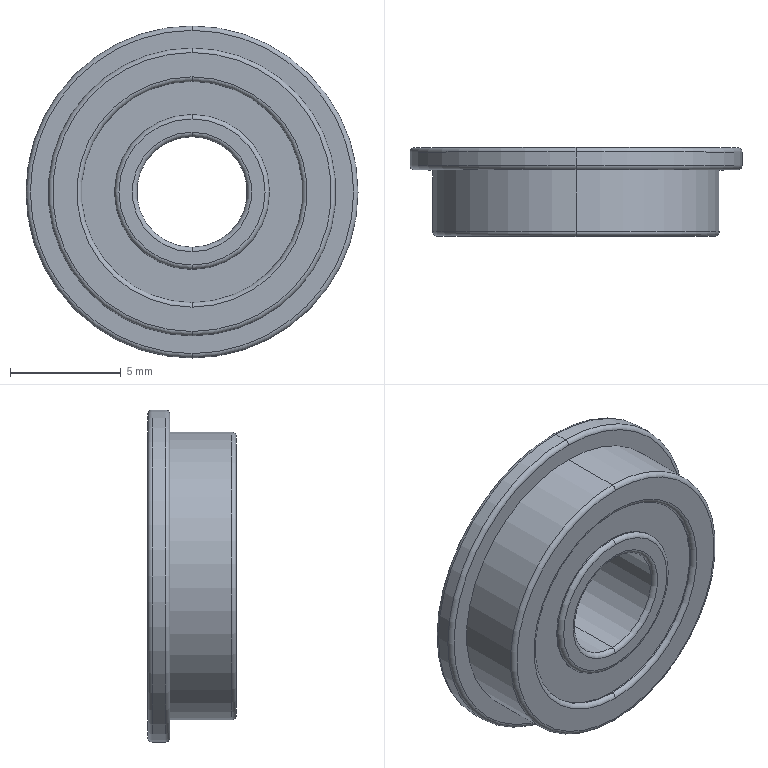Part | NX | features BREP 1 | 1 solid | 39 faces | box 15 x 4 x 15 mm | volume 474 mm3 | torus 18 | cylinder 14 | plane 7 | commonest cylinder face diameters 7 x4 10 x4 5 x2 13 x2 15 x2
STEP:
#1=CARTESIAN_POINT('',(0.,3.8,2.5));
#2=VERTEX_POINT('',#1);
#3=CARTESIAN_POINT('',(0.,4.,2.7));
#4=VERTEX_POINT('',#3);
#5=CARTESIAN_POINT('',(0.,3.8,2.7));
#6=DIRECTION('',(1.,0.,0.));
#7=DIRECTION('',(0.,0.,-1.));
#8=AXIS2_PLACEMENT_3D('',#5,#6,#7);
#9=CIRCLE('',#8,0.2);
#10=EDGE_CURVE('',#2,#4,#9,.T.);
#11=ORIENTED_EDGE('',*,*,#10,.F.);
#12=CARTESIAN_POINT('',(0.,3.8,-2.5));
#13=VERTEX_POINT('',#12);
#14=CARTESIAN_POINT('',(0.,3.8,0.));
#15=DIRECTION('',(0.,1.,0.));
#16=DIRECTION('',(0.,0.,-1.));
#17=AXIS2_PLACEMENT_3D('',#14,#15,#16);
#18=CIRCLE('',#17,2.5);
#19=EDGE_CURVE('',#13,#2,#18,.T.);
#20=ORIENTED_EDGE('',*,*,#19,.F.);
#21=CARTESIAN_POINT('',(0.,4.,-2.7));
#22=VERTEX_POINT('',#21);
#23=CARTESIAN_POINT('',(0.,3.8,-2.7));
#24=DIRECTION('',(-1.,0.,0.));
#25=DIRECTION('',(0.,0.,1.));
#26=AXIS2_PLACEMENT_3D('',#23,#24,#25);
#27=CIRCLE('',#26,0.2);
#28=EDGE_CURVE('',#13,#22,#27,.T.);
#29=ORIENTED_EDGE('',*,*,#28,.T.);
#30=CARTESIAN_POINT('',(0.,4.,0.));
#31=DIRECTION('',(0.,-1.,0.));
#32=DIRECTION('',(0.,0.,-1.));
#33=AXIS2_PLACEMENT_3D('',#30,#31,#32);
#34=CIRCLE('',#33,2.7);
#35=EDGE_CURVE('',#4,#22,#34,.T.);
#36=ORIENTED_EDGE('',*,*,#35,.F.);
#37=EDGE_LOOP('',(#11,#20,#29,#36));
#38=FACE_BOUND('',#37,.T.);
#39=CARTESIAN_POINT('',(0.,3.8,0.));
#40=DIRECTION('',(0.,-1.,0.));
#41=DIRECTION('',(0.,0.,-1.));
#42=AXIS2_PLACEMENT_3D('',#39,#40,#41);
#43=TOROIDAL_SURFACE('',#42,2.7,0.2);
#44=ADVANCED_FACE('',(#38),#43,.T.);
#45=CARTESIAN_POINT('',(0.,4.,3.3));
#46=VERTEX_POINT('',#45);
#47=CARTESIAN_POINT('',(0.,3.8,3.5));
#48=VERTEX_POINT('',#47);
#49=CARTESIAN_POINT('',(0.,3.8,3.3));
#50=DIRECTION('',(1.,0.,0.));
#51=DIRECTION('',(0.,0.,-1.));
#52=AXIS2_PLACEMENT_3D('',#49,#50,#51);
#53=CIRCLE('',#52,0.2);
#54=EDGE_CURVE('',#46,#48,#53,.T.);
#55=ORIENTED_EDGE('',*,*,#54,.F.);
#56=CARTESIAN_POINT('',(0.,4.,-3.3));
#57=VERTEX_POINT('',#56);
#58=CARTESIAN_POINT('',(0.,4.,0.));
#59=DIRECTION('',(0.,1.,0.));
#60=DIRECTION('',(0.,0.,-1.));
#61=AXIS2_PLACEMENT_3D('',#58,#59,#60);
#62=CIRCLE('',#61,3.3);
#63=EDGE_CURVE('',#57,#46,#62,.T.);
#64=ORIENTED_EDGE('',*,*,#63,.F.);
#65=CARTESIAN_POINT('',(0.,3.8,-3.5));
#66=VERTEX_POINT('',#65);
#67=CARTESIAN_POINT('',(0.,3.8,-3.3));
#68=DIRECTION('',(-1.,0.,0.));
#69=DIRECTION('',(0.,0.,1.));
#70=AXIS2_PLACEMENT_3D('',#67,#68,#69);
#71=CIRCLE('',#70,0.2);
#72=EDGE_CURVE('',#57,#66,#71,.T.);
#73=ORIENTED_EDGE('',*,*,#72,.T.);
#74=CARTESIAN_POINT('',(0.,3.8,0.));
#75=DIRECTION('',(0.,-1.,0.));
#76=DIRECTION('',(0.,0.,-1.));
#77=AXIS2_PLACEMENT_3D('',#74,#75,#76);
#78=CIRCLE('',#77,3.5);
#79=EDGE_CURVE('',#48,#66,#78,.T.);
#80=ORIENTED_EDGE('',*,*,#79,.F.);
#81=EDGE_LOOP('',(#55,#64,#73,#80));
#82=FACE_BOUND('',#81,.T.);
#83=CARTESIAN_POINT('',(0.,3.8,0.));
#84=DIRECTION('',(0.,-1.,0.));
#85=DIRECTION('',(0.,0.,-1.));
#86=AXIS2_PLACEMENT_3D('',#83,#84,#85);
#87=TOROIDAL_SURFACE('',#86,3.3,0.2);
#88=ADVANCED_FACE('',(#82),#87,.T.);
#89=CARTESIAN_POINT('',(0.,3.8,5.));
#90=VERTEX_POINT('',#89);
#91=CARTESIAN_POINT('',(0.,4.,5.2));
#92=VERTEX_POINT('',#91);
#93=CARTESIAN_POINT('',(0.,3.8,5.2));
#94=DIRECTION('',(1.,0.,0.));
#95=DIRECTION('',(0.,0.,-1.));
#96=AXIS2_PLACEMENT_3D('',#93,#94,#95);
#97=CIRCLE('',#96,0.2);
#98=EDGE_CURVE('',#90,#92,#97,.T.);
#99=ORIENTED_EDGE('',*,*,#98,.F.);
#100=CARTESIAN_POINT('',(0.,3.8,-5.));
#101=VERTEX_POINT('',#100);
#102=CARTESIAN_POINT('',(0.,3.8,0.));
#103=DIRECTION('',(0.,1.,0.));
#104=DIRECTION('',(0.,0.,-1.));
#105=AXIS2_PLACEMENT_3D('',#102,#103,#104);
#106=CIRCLE('',#105,5.);
#107=EDGE_CURVE('',#101,#90,#106,.T.);
#108=ORIENTED_EDGE('',*,*,#107,.F.);
#109=CARTESIAN_POINT('',(0.,4.,-5.2));
#110=VERTEX_POINT('',#109);
#111=CARTESIAN_POINT('',(0.,3.8,-5.2));
#112=DIRECTION('',(-1.,0.,0.));
#113=DIRECTION('',(0.,0.,1.));
#114=AXIS2_PLACEMENT_3D('',#111,#112,#113);
#115=CIRCLE('',#114,0.2);
#116=EDGE_CURVE('',#101,#110,#115,.T.);
#117=ORIENTED_EDGE('',*,*,#116,.T.);
#118=CARTESIAN_POINT('',(0.,4.,0.));
#119=DIRECTION('',(0.,-1.,0.));
#120=DIRECTION('',(0.,0.,-1.));
#121=AXIS2_PLACEMENT_3D('',#118,#119,#120);
#122=CIRCLE('',#121,5.2);
#123=EDGE_CURVE('',#92,#110,#122,.T.);
#124=ORIENTED_EDGE('',*,*,#123,.F.);
#125=EDGE_LOOP('',(#99,#108,#117,#124));
#126=FACE_BOUND('',#125,.T.);
#127=CARTESIAN_POINT('',(0.,3.8,0.));
#128=DIRECTION('',(0.,-1.,0.));
#129=DIRECTION('',(0.,0.,-1.));
#130=AXIS2_PLACEMENT_3D('',#127,#128,#129);
#131=TOROIDAL_SURFACE('',#130,5.2,0.2);
#132=ADVANCED_FACE('',(#126),#131,.T.);
#133=CARTESIAN_POINT('',(0.,4.,7.3));
#134=VERTEX_POINT('',#133);
#135=CARTESIAN_POINT('',(0.,3.8,7.5));
#136=VERTEX_POINT('',#135);
#137=CARTESIAN_POINT('',(0.,3.8,7.3));
#138=DIRECTION('',(1.,0.,0.));
#139=DIRECTION('',(0.,0.,-1.));
#140=AXIS2_PLACEMENT_3D('',#137,#138,#139);
#141=CIRCLE('',#140,0.2);
#142=EDGE_CURVE('',#134,#136,#141,.T.);
#143=ORIENTED_EDGE('',*,*,#142,.F.);
#144=CARTESIAN_POINT('',(0.,4.,-7.3));
#145=VERTEX_POINT('',#144);
#146=CARTESIAN_POINT('',(0.,4.,0.));
#147=DIRECTION('',(0.,1.,0.));
#148=DIRECTION('',(0.,0.,-1.));
#149=AXIS2_PLACEMENT_3D('',#146,#147,#148);
#150=CIRCLE('',#149,7.3);
#151=EDGE_CURVE('',#145,#134,#150,.T.);
#152=ORIENTED_EDGE('',*,*,#151,.F.);
#153=CARTESIAN_POINT('',(0.,3.8,-7.5));
#154=VERTEX_POINT('',#153);
#155=CARTESIAN_POINT('',(0.,3.8,-7.3));
#156=DIRECTION('',(-1.,0.,0.));
#157=DIRECTION('',(0.,0.,1.));
#158=AXIS2_PLACEMENT_3D('',#155,#156,#157);
#159=CIRCLE('',#158,0.2);
#160=EDGE_CURVE('',#145,#154,#159,.T.);
#161=ORIENTED_EDGE('',*,*,#160,.T.);
#162=CARTESIAN_POINT('',(0.,3.8,0.));
#163=DIRECTION('',(0.,-1.,0.));
#164=DIRECTION('',(0.,0.,-1.));
#165=AXIS2_PLACEMENT_3D('',#162,#163,#164);
#166=CIRCLE('',#165,7.5);
#167=EDGE_CURVE('',#136,#154,#166,.T.);
#168=ORIENTED_EDGE('',*,*,#167,.F.);
#169=EDGE_LOOP('',(#143,#152,#161,#168));
#170=FACE_BOUND('',#169,.T.);
#171=CARTESIAN_POINT('',(0.,3.8,0.));
#172=DIRECTION('',(0.,-1.,0.));
#173=DIRECTION('',(0.,0.,-1.));
#174=AXIS2_PLACEMENT_3D('',#171,#172,#173);
#175=TOROIDAL_SURFACE('',#174,7.3,0.2);
#176=ADVANCED_FACE('',(#170),#175,.T.);
#177=CARTESIAN_POINT('',(0.,3.2,-7.5));
#178=VERTEX_POINT('',#177);
#179=CARTESIAN_POINT('',(0.,3.,-7.3));
#180=VERTEX_POINT('',#179);
#181=CARTESIAN_POINT('',(0.,3.2,-7.3));
#182=DIRECTION('',(1.,0.,0.));
#183=DIRECTION('',(0.,0.,-1.));
#184=AXIS2_PLACEMENT_3D('',#181,#182,#183);
#185=CIRCLE('',#184,0.2);
#186=EDGE_CURVE('',#178,#180,#185,.F.);
#187=ORIENTED_EDGE('',*,*,#186,.T.);
#188=CARTESIAN_POINT('',(0.,3.,7.3));
#189=VERTEX_POINT('',#188);
#190=CARTESIAN_POINT('',(0.,3.,0.));
#191=DIRECTION('',(0.,-1.,0.));
#192=DIRECTION('',(0.,0.,1.));
#193=AXIS2_PLACEMENT_3D('',#190,#191,#192);
#194=CIRCLE('',#193,7.3);
#195=EDGE_CURVE('',#189,#180,#194,.T.);
#196=ORIENTED_EDGE('',*,*,#195,.F.);
#197=CARTESIAN_POINT('',(0.,3.2,7.5));
#198=VERTEX_POINT('',#197);
#199=CARTESIAN_POINT('',(0.,3.2,7.3));
#200=DIRECTION('',(-1.,0.,0.));
#201=DIRECTION('',(0.,0.,1.));
#202=AXIS2_PLACEMENT_3D('',#199,#200,#201);
#203=CIRCLE('',#202,0.2);
#204=EDGE_CURVE('',#198,#189,#203,.F.);
#205=ORIENTED_EDGE('',*,*,#204,.F.);
#206=CARTESIAN_POINT('',(0.,3.2,0.));
#207=DIRECTION('',(0.,1.,0.));
#208=DIRECTION('',(0.,0.,1.));
#209=AXIS2_PLACEMENT_3D('',#206,#207,#208);
#210=CIRCLE('',#209,7.5);
#211=EDGE_CURVE('',#178,#198,#210,.T.);
#212=ORIENTED_EDGE('',*,*,#211,.F.);
#213=EDGE_LOOP('',(#187,#196,#205,#212));
#214=FACE_BOUND('',#213,.T.);
#215=CARTESIAN_POINT('',(0.,3.2,0.));
#216=DIRECTION('',(0.,1.,0.));
#217=DIRECTION('',(0.,0.,1.));
#218=AXIS2_PLACEMENT_3D('',#215,#216,#217);
#219=TOROIDAL_SURFACE('',#218,7.3,0.2);
#220=ADVANCED_FACE('',(#214),#219,.T.);
#221=CARTESIAN_POINT('',(0.,0.2,-6.5));
#222=VERTEX_POINT('',#221);
#223=CARTESIAN_POINT('',(0.,0.,-6.3));
#224=VERTEX_POINT('',#223);
#225=CARTESIAN_POINT('',(0.,0.2,-6.3));
#226=DIRECTION('',(1.,0.,0.));
#227=DIRECTION('',(0.,0.,-1.));
#228=AXIS2_PLACEMENT_3D('',#225,#226,#227);
#229=CIRCLE('',#228,0.2);
#230=EDGE_CURVE('',#222,#224,#229,.F.);
#231=ORIENTED_EDGE('',*,*,#230,.T.);
#232=CARTESIAN_POINT('',(0.,0.,6.3));
#233=VERTEX_POINT('',#232);
#234=CARTESIAN_POINT('',(0.,0.,0.));
#235=DIRECTION('',(0.,-1.,0.));
#236=DIRECTION('',(0.,0.,1.));
#237=AXIS2_PLACEMENT_3D('',#234,#235,#236);
#238=CIRCLE('',#237,6.3);
#239=EDGE_CURVE('',#233,#224,#238,.T.);
#240=ORIENTED_EDGE('',*,*,#239,.F.);
#241=CARTESIAN_POINT('',(0.,0.2,6.5));
#242=VERTEX_POINT('',#241);
#243=CARTESIAN_POINT('',(0.,0.2,6.3));
#244=DIRECTION('',(-1.,0.,0.));
#245=DIRECTION('',(0.,0.,1.));
#246=AXIS2_PLACEMENT_3D('',#243,#244,#245);
#247=CIRCLE('',#246,0.2);
#248=EDGE_CURVE('',#242,#233,#247,.F.);
#249=ORIENTED_EDGE('',*,*,#248,.F.);
#250=CARTESIAN_POINT('',(0.,0.2,0.));
#251=DIRECTION('',(0.,1.,0.));
#252=DIRECTION('',(0.,0.,1.));
#253=AXIS2_PLACEMENT_3D('',#250,#251,#252);
#254=CIRCLE('',#253,6.5);
#255=EDGE_CURVE('',#222,#242,#254,.T.);
#256=ORIENTED_EDGE('',*,*,#255,.F.);
#257=EDGE_LOOP('',(#231,#240,#249,#256));
#258=FACE_BOUND('',#257,.T.);
#259=CARTESIAN_POINT('',(0.,0.2,0.));
#260=DIRECTION('',(0.,1.,0.));
#261=DIRECTION('',(0.,0.,1.));
#262=AXIS2_PLACEMENT_3D('',#259,#260,#261);
#263=TOROIDAL_SURFACE('',#262,6.3,0.2);
#264=ADVANCED_FACE('',(#258),#263,.T.);
#265=CARTESIAN_POINT('',(0.,0.,-5.2));
#266=VERTEX_POINT('',#265);
#267=CARTESIAN_POINT('',(0.,0.2,-5.));
#268=VERTEX_POINT('',#267);
#269=CARTESIAN_POINT('',(0.,0.2,-5.2));
#270=DIRECTION('',(1.,0.,0.));
#271=DIRECTION('',(0.,0.,-1.));
#272=AXIS2_PLACEMENT_3D('',#269,#270,#271);
#273=CIRCLE('',#272,0.2);
#274=EDGE_CURVE('',#266,#268,#273,.F.);
#275=ORIENTED_EDGE('',*,*,#274,.T.);
#276=CARTESIAN_POINT('',(0.,0.2,5.));
#277=VERTEX_POINT('',#276);
#278=CARTESIAN_POINT('',(0.,0.2,0.));
#279=DIRECTION('',(0.,-1.,0.));
#280=DIRECTION('',(0.,0.,1.));
#281=AXIS2_PLACEMENT_3D('',#278,#279,#280);
#282=CIRCLE('',#281,5.);
#283=EDGE_CURVE('',#277,#268,#282,.T.);
#284=ORIENTED_EDGE('',*,*,#283,.F.);
#285=CARTESIAN_POINT('',(0.,0.,5.2));
#286=VERTEX_POINT('',#285);
#287=CARTESIAN_POINT('',(0.,0.2,5.2));
#288=DIRECTION('',(-1.,0.,0.));
#289=DIRECTION('',(0.,0.,1.));
#290=AXIS2_PLACEMENT_3D('',#287,#288,#289);
#291=CIRCLE('',#290,0.2);
#292=EDGE_CURVE('',#286,#277,#291,.F.);
#293=ORIENTED_EDGE('',*,*,#292,.F.);
#294=CARTESIAN_POINT('',(0.,0.,0.));
#295=DIRECTION('',(0.,1.,0.));
#296=DIRECTION('',(0.,0.,1.));
#297=AXIS2_PLACEMENT_3D('',#294,#295,#296);
#298=CIRCLE('',#297,5.2);
#299=EDGE_CURVE('',#266,#286,#298,.T.);
#300=ORIENTED_EDGE('',*,*,#299,.F.);
#301=EDGE_LOOP('',(#275,#284,#293,#300));
#302=FACE_BOUND('',#301,.T.);
#303=CARTESIAN_POINT('',(0.,0.2,0.));
#304=DIRECTION('',(0.,1.,0.));
#305=DIRECTION('',(0.,0.,1.));
#306=AXIS2_PLACEMENT_3D('',#303,#304,#305);
#307=TOROIDAL_SURFACE('',#306,5.2,0.2);
#308=ADVANCED_FACE('',(#302),#307,.T.);
#309=CARTESIAN_POINT('',(0.,0.2,-3.5));
#310=VERTEX_POINT('',#309);
#311=CARTESIAN_POINT('',(0.,0.,-3.3));
#312=VERTEX_POINT('',#311);
#313=CARTESIAN_POINT('',(0.,0.2,-3.3));
#314=DIRECTION('',(1.,0.,0.));
#315=DIRECTION('',(0.,0.,-1.));
#316=AXIS2_PLACEMENT_3D('',#313,#314,#315);
#317=CIRCLE('',#316,0.2);
#318=EDGE_CURVE('',#310,#312,#317,.F.);
#319=ORIENTED_EDGE('',*,*,#318,.T.);
#320=CARTESIAN_POINT('',(0.,0.,3.3));
#321=VERTEX_POINT('',#320);
#322=CARTESIAN_POINT('',(0.,0.,0.));
#323=DIRECTION('',(0.,-1.,0.));
#324=DIRECTION('',(0.,0.,1.));
#325=AXIS2_PLACEMENT_3D('',#322,#323,#324);
#326=CIRCLE('',#325,3.3);
#327=EDGE_CURVE('',#321,#312,#326,.T.);
#328=ORIENTED_EDGE('',*,*,#327,.F.);
#329=CARTESIAN_POINT('',(0.,0.2,3.5));
#330=VERTEX_POINT('',#329);
#331=CARTESIAN_POINT('',(0.,0.2,3.3));
#332=DIRECTION('',(-1.,0.,0.));
#333=DIRECTION('',(0.,0.,1.));
#334=AXIS2_PLACEMENT_3D('',#331,#332,#333);
#335=CIRCLE('',#334,0.2);
#336=EDGE_CURVE('',#330,#321,#335,.F.);
#337=ORIENTED_EDGE('',*,*,#336,.F.);
#338=CARTESIAN_POINT('',(0.,0.2,0.));
#339=DIRECTION('',(0.,1.,0.));
#340=DIRECTION('',(0.,0.,1.));
#341=AXIS2_PLACEMENT_3D('',#338,#339,#340);
#342=CIRCLE('',#341,3.5);
#343=EDGE_CURVE('',#310,#330,#342,.T.);
#344=ORIENTED_EDGE('',*,*,#343,.F.);
#345=EDGE_LOOP('',(#319,#328,#337,#344));
#346=FACE_BOUND('',#345,.T.);
#347=CARTESIAN_POINT('',(0.,0.2,0.));
#348=DIRECTION('',(0.,1.,0.));
#349=DIRECTION('',(0.,0.,1.));
#350=AXIS2_PLACEMENT_3D('',#347,#348,#349);
#351=TOROIDAL_SURFACE('',#350,3.3,0.2);
#352=ADVANCED_FACE('',(#346),#351,.T.);
#353=CARTESIAN_POINT('',(0.,0.,-2.7));
#354=VERTEX_POINT('',#353);
#355=CARTESIAN_POINT('',(0.,0.2,-2.5));
#356=VERTEX_POINT('',#355);
#357=CARTESIAN_POINT('',(0.,0.2,-2.7));
#358=DIRECTION('',(1.,0.,0.));
#359=DIRECTION('',(0.,0.,-1.));
#360=AXIS2_PLACEMENT_3D('',#357,#358,#359);
#361=CIRCLE('',#360,0.2);
#362=EDGE_CURVE('',#354,#356,#361,.F.);
#363=ORIENTED_EDGE('',*,*,#362,.T.);
#364=CARTESIAN_POINT('',(0.,0.2,2.5));
#365=VERTEX_POINT('',#364);
#366=CARTESIAN_POINT('',(0.,0.2,0.));
#367=DIRECTION('',(0.,-1.,0.));
#368=DIRECTION('',(0.,0.,1.));
#369=AXIS2_PLACEMENT_3D('',#366,#367,#368);
#370=CIRCLE('',#369,2.5);
#371=EDGE_CURVE('',#365,#356,#370,.T.);
#372=ORIENTED_EDGE('',*,*,#371,.F.);
#373=CARTESIAN_POINT('',(0.,0.,2.7));
#374=VERTEX_POINT('',#373);
#375=CARTESIAN_POINT('',(0.,0.2,2.7));
#376=DIRECTION('',(-1.,0.,0.));
#377=DIRECTION('',(0.,0.,1.));
#378=AXIS2_PLACEMENT_3D('',#375,#376,#377);
#379=CIRCLE('',#378,0.2);
#380=EDGE_CURVE('',#374,#365,#379,.F.);
#381=ORIENTED_EDGE('',*,*,#380,.F.);
#382=CARTESIAN_POINT('',(0.,0.,0.));
#383=DIRECTION('',(0.,1.,0.));
#384=DIRECTION('',(0.,0.,1.));
#385=AXIS2_PLACEMENT_3D('',#382,#383,#384);
#386=CIRCLE('',#385,2.7);
#387=EDGE_CURVE('',#354,#374,#386,.T.);
#388=ORIENTED_EDGE('',*,*,#387,.F.);
#389=EDGE_LOOP('',(#363,#372,#381,#388));
#390=FACE_BOUND('',#389,.T.);
#391=CARTESIAN_POINT('',(0.,0.2,0.));
#392=DIRECTION('',(0.,1.,0.));
#393=DIRECTION('',(0.,0.,1.));
#394=AXIS2_PLACEMENT_3D('',#391,#392,#393);
#395=TOROIDAL_SURFACE('',#394,2.7,0.2);
#396=ADVANCED_FACE('',(#390),#395,.T.);
#397=CARTESIAN_POINT('',(0.,0.25,3.5));
#398=VERTEX_POINT('',#397);
#399=CARTESIAN_POINT('',(0.,0.,3.5));
#400=DIRECTION('',(0.,-1.,0.));
#401=VECTOR('',#400,1000.);
#402=LINE('',#399,#401);
#403=EDGE_CURVE('',#398,#330,#402,.T.);
#404=ORIENTED_EDGE('',*,*,#403,.F.);
#405=CARTESIAN_POINT('',(0.,0.25,-3.5));
#406=VERTEX_POINT('',#405);
#407=CARTESIAN_POINT('',(0.,0.25,0.));
#408=DIRECTION('',(0.,-1.,0.));
#409=DIRECTION('',(0.,0.,-1.));
#410=AXIS2_PLACEMENT_3D('',#407,#408,#409);
#411=CIRCLE('',#410,3.5);
#412=EDGE_CURVE('',#398,#406,#411,.T.);
#413=ORIENTED_EDGE('',*,*,#412,.T.);
#414=CARTESIAN_POINT('',(0.,0.,-3.5));
#415=DIRECTION('',(0.,-1.,0.));
#416=VECTOR('',#415,1000.);
#417=LINE('',#414,#416);
#418=EDGE_CURVE('',#406,#310,#417,.T.);
#419=ORIENTED_EDGE('',*,*,#418,.T.);
#420=ORIENTED_EDGE('',*,*,#343,.T.);
#421=EDGE_LOOP('',(#404,#413,#419,#420));
#422=FACE_BOUND('',#421,.T.);
#423=CARTESIAN_POINT('',(0.,0.,0.));
#424=DIRECTION('',(0.,-1.,0.));
#425=DIRECTION('',(0.,0.,-1.));
#426=AXIS2_PLACEMENT_3D('',#423,#424,#425);
#427=CYLINDRICAL_SURFACE('',#426,3.5);
#428=ADVANCED_FACE('',(#422),#427,.T.);
#429=CARTESIAN_POINT('',(0.,0.25,-5.));
#430=VERTEX_POINT('',#429);
#431=CARTESIAN_POINT('',(0.,0.25,5.));
#432=VERTEX_POINT('',#431);
#433=CARTESIAN_POINT('',(0.,0.25,0.));
#434=DIRECTION('',(0.,-1.,0.));
#435=DIRECTION('',(0.,0.,-1.));
#436=AXIS2_PLACEMENT_3D('',#433,#434,#435);
#437=CIRCLE('',#436,5.);
#438=EDGE_CURVE('',#430,#432,#437,.T.);
#439=ORIENTED_EDGE('',*,*,#438,.T.);
#440=CARTESIAN_POINT('',(0.,0.25,0.));
#441=DIRECTION('',(0.,-1.,0.));
#442=DIRECTION('',(0.,0.,-1.));
#443=AXIS2_PLACEMENT_3D('',#440,#441,#442);
#444=CIRCLE('',#443,5.);
#445=EDGE_CURVE('',#432,#430,#444,.T.);
#446=ORIENTED_EDGE('',*,*,#445,.T.);
#447=EDGE_LOOP('',(#439,#446));
#448=FACE_BOUND('',#447,.T.);
#449=CARTESIAN_POINT('',(0.,0.25,0.));
#450=DIRECTION('',(0.,-1.,0.));
#451=DIRECTION('',(0.,0.,-1.));
#452=AXIS2_PLACEMENT_3D('',#449,#450,#451);
#453=CIRCLE('',#452,3.5);
#454=EDGE_CURVE('',#406,#398,#453,.T.);
#455=ORIENTED_EDGE('',*,*,#454,.F.);
#456=ORIENTED_EDGE('',*,*,#412,.F.);
#457=EDGE_LOOP('',(#455,#456));
#458=FACE_BOUND('',#457,.T.);
#459=CARTESIAN_POINT('',(-3.5,0.25,0.));
#460=DIRECTION('',(0.,1.,0.));
#461=DIRECTION('',(0.,0.,1.));
#462=AXIS2_PLACEMENT_3D('',#459,#460,#461);
#463=PLANE('',#462);
#464=ADVANCED_FACE('',(#448,#458),#463,.F.);
#465=CARTESIAN_POINT('',(0.,0.,5.));
#466=DIRECTION('',(0.,-1.,0.));
#467=VECTOR('',#466,1000.);
#468=LINE('',#465,#467);
#469=EDGE_CURVE('',#432,#277,#468,.T.);
#470=ORIENTED_EDGE('',*,*,#469,.F.);
#471=ORIENTED_EDGE('',*,*,#438,.F.);
#472=CARTESIAN_POINT('',(0.,0.,-5.));
#473=DIRECTION('',(0.,-1.,0.));
#474=VECTOR('',#473,1000.);
#475=LINE('',#472,#474);
#476=EDGE_CURVE('',#430,#268,#475,.T.);
#477=ORIENTED_EDGE('',*,*,#476,.T.);
#478=CARTESIAN_POINT('',(0.,0.2,0.));
#479=DIRECTION('',(0.,-1.,0.));
#480=DIRECTION('',(0.,0.,1.));
#481=AXIS2_PLACEMENT_3D('',#478,#479,#480);
#482=CIRCLE('',#481,5.);
#483=EDGE_CURVE('',#268,#277,#482,.T.);
#484=ORIENTED_EDGE('',*,*,#483,.T.);
#485=EDGE_LOOP('',(#470,#471,#477,#484));
#486=FACE_BOUND('',#485,.T.);
#487=CARTESIAN_POINT('',(0.,0.,0.));
#488=DIRECTION('',(0.,-1.,0.));
#489=DIRECTION('',(0.,0.,-1.));
#490=AXIS2_PLACEMENT_3D('',#487,#488,#489);
#491=CYLINDRICAL_SURFACE('',#490,5.);
#492=ADVANCED_FACE('',(#486),#491,.F.);
#493=ORIENTED_EDGE('',*,*,#239,.T.);
#494=CARTESIAN_POINT('',(0.,0.,0.));
#495=DIRECTION('',(0.,-1.,0.));
#496=DIRECTION('',(0.,0.,1.));
#497=AXIS2_PLACEMENT_3D('',#494,#495,#496);
#498=CIRCLE('',#497,6.3);
#499=EDGE_CURVE('',#224,#233,#498,.T.);
#500=ORIENTED_EDGE('',*,*,#499,.T.);
#501=EDGE_LOOP('',(#493,#500));
#502=FACE_BOUND('',#501,.T.);
#503=CARTESIAN_POINT('',(0.,0.,0.));
#504=DIRECTION('',(0.,1.,0.));
#505=DIRECTION('',(0.,0.,1.));
#506=AXIS2_PLACEMENT_3D('',#503,#504,#505);
#507=CIRCLE('',#506,5.2);
#508=EDGE_CURVE('',#286,#266,#507,.T.);
#509=ORIENTED_EDGE('',*,*,#508,.T.);
#510=ORIENTED_EDGE('',*,*,#299,.T.);
#511=EDGE_LOOP('',(#509,#510));
#512=FACE_BOUND('',#511,.T.);
#513=CARTESIAN_POINT('',(-6.5,0.,0.));
#514=DIRECTION('',(0.,1.,0.));
#515=DIRECTION('',(0.,0.,1.));
#516=AXIS2_PLACEMENT_3D('',#513,#514,#515);
#517=PLANE('',#516);
#518=ADVANCED_FACE('',(#502,#512),#517,.F.);
#519=CARTESIAN_POINT('',(0.,3.,6.5));
#520=VERTEX_POINT('',#519);
#521=CARTESIAN_POINT('',(0.,0.,6.5));
#522=DIRECTION('',(0.,-1.,0.));
#523=VECTOR('',#522,1000.);
#524=LINE('',#521,#523);
#525=EDGE_CURVE('',#520,#242,#524,.T.);
#526=ORIENTED_EDGE('',*,*,#525,.F.);
#527=CARTESIAN_POINT('',(0.,3.,-6.5));
#528=VERTEX_POINT('',#527);
#529=CARTESIAN_POINT('',(0.,3.,0.));
#530=DIRECTION('',(0.,-1.,0.));
#531=DIRECTION('',(0.,0.,-1.));
#532=AXIS2_PLACEMENT_3D('',#529,#530,#531);
#533=CIRCLE('',#532,6.5);
#534=EDGE_CURVE('',#520,#528,#533,.T.);
#535=ORIENTED_EDGE('',*,*,#534,.T.);
#536=CARTESIAN_POINT('',(0.,0.,-6.5));
#537=DIRECTION('',(0.,-1.,0.));
#538=VECTOR('',#537,1000.);
#539=LINE('',#536,#538);
#540=EDGE_CURVE('',#528,#222,#539,.T.);
#541=ORIENTED_EDGE('',*,*,#540,.T.);
#542=ORIENTED_EDGE('',*,*,#255,.T.);
#543=EDGE_LOOP('',(#526,#535,#541,#542));
#544=FACE_BOUND('',#543,.T.);
#545=CARTESIAN_POINT('',(0.,0.,0.));
#546=DIRECTION('',(0.,-1.,0.));
#547=DIRECTION('',(0.,0.,-1.));
#548=AXIS2_PLACEMENT_3D('',#545,#546,#547);
#549=CYLINDRICAL_SURFACE('',#548,6.5);
#550=ADVANCED_FACE('',(#544),#549,.T.);
#551=CARTESIAN_POINT('',(0.,3.,0.));
#552=DIRECTION('',(0.,-1.,0.));
#553=DIRECTION('',(0.,0.,-1.));
#554=AXIS2_PLACEMENT_3D('',#551,#552,#553);
#555=CIRCLE('',#554,6.5);
#556=EDGE_CURVE('',#528,#520,#555,.T.);
#557=ORIENTED_EDGE('',*,*,#556,.F.);
#558=ORIENTED_EDGE('',*,*,#534,.F.);
#559=EDGE_LOOP('',(#557,#558));
#560=FACE_BOUND('',#559,.T.);
#561=ORIENTED_EDGE('',*,*,#195,.T.);
#562=CARTESIAN_POINT('',(0.,3.,0.));
#563=DIRECTION('',(0.,-1.,0.));
#564=DIRECTION('',(0.,0.,1.));
#565=AXIS2_PLACEMENT_3D('',#562,#563,#564);
#566=CIRCLE('',#565,7.3);
#567=EDGE_CURVE('',#180,#189,#566,.T.);
#568=ORIENTED_EDGE('',*,*,#567,.T.);
#569=EDGE_LOOP('',(#561,#568));
#570=FACE_BOUND('',#569,.T.);
#571=CARTESIAN_POINT('',(-7.5,3.,0.));
#572=DIRECTION('',(0.,1.,0.));
#573=DIRECTION('',(0.,0.,1.));
#574=AXIS2_PLACEMENT_3D('',#571,#572,#573);
#575=PLANE('',#574);
#576=ADVANCED_FACE('',(#560,#570),#575,.F.);
#577=CARTESIAN_POINT('',(0.,0.,7.5));
#578=DIRECTION('',(0.,-1.,0.));
#579=VECTOR('',#578,1000.);
#580=LINE('',#577,#579);
#581=EDGE_CURVE('',#136,#198,#580,.T.);
#582=ORIENTED_EDGE('',*,*,#581,.F.);
#583=ORIENTED_EDGE('',*,*,#167,.T.);
#584=CARTESIAN_POINT('',(0.,0.,-7.5));
#585=DIRECTION('',(0.,-1.,0.));
#586=VECTOR('',#585,1000.);
#587=LINE('',#584,#586);
#588=EDGE_CURVE('',#154,#178,#587,.T.);
#589=ORIENTED_EDGE('',*,*,#588,.T.);
#590=ORIENTED_EDGE('',*,*,#211,.T.);
#591=EDGE_LOOP('',(#582,#583,#589,#590));
#592=FACE_BOUND('',#591,.T.);
#593=CARTESIAN_POINT('',(0.,0.,0.));
#594=DIRECTION('',(0.,-1.,0.));
#595=DIRECTION('',(0.,0.,-1.));
#596=AXIS2_PLACEMENT_3D('',#593,#594,#595);
#597=CYLINDRICAL_SURFACE('',#596,7.5);
#598=ADVANCED_FACE('',(#592),#597,.T.);
#599=CARTESIAN_POINT('',(0.,4.,0.));
#600=DIRECTION('',(0.,-1.,0.));
#601=DIRECTION('',(0.,0.,-1.));
#602=AXIS2_PLACEMENT_3D('',#599,#600,#601);
#603=CIRCLE('',#602,5.2);
#604=EDGE_CURVE('',#110,#92,#603,.T.);
#605=ORIENTED_EDGE('',*,*,#604,.T.);
#606=ORIENTED_EDGE('',*,*,#123,.T.);
#607=EDGE_LOOP('',(#605,#606));
#608=FACE_BOUND('',#607,.T.);
#609=ORIENTED_EDGE('',*,*,#151,.T.);
#610=CARTESIAN_POINT('',(0.,4.,0.));
#611=DIRECTION('',(0.,1.,0.));
#612=DIRECTION('',(0.,0.,-1.));
#613=AXIS2_PLACEMENT_3D('',#610,#611,#612);
#614=CIRCLE('',#613,7.3);
#615=EDGE_CURVE('',#134,#145,#614,.T.);
#616=ORIENTED_EDGE('',*,*,#615,.T.);
#617=EDGE_LOOP('',(#609,#616));
#618=FACE_BOUND('',#617,.T.);
#619=CARTESIAN_POINT('',(-5.,4.,0.));
#620=DIRECTION('',(0.,-1.,0.));
#621=DIRECTION('',(0.,0.,-1.));
#622=AXIS2_PLACEMENT_3D('',#619,#620,#621);
#623=PLANE('',#622);
#624=ADVANCED_FACE('',(#608,#618),#623,.F.);
#625=CARTESIAN_POINT('',(0.,3.75,5.));
#626=VERTEX_POINT('',#625);
#627=CARTESIAN_POINT('',(0.,0.,5.));
#628=DIRECTION('',(0.,-1.,0.));
#629=VECTOR('',#628,1000.);
#630=LINE('',#627,#629);
#631=EDGE_CURVE('',#90,#626,#630,.T.);
#632=ORIENTED_EDGE('',*,*,#631,.F.);
#633=CARTESIAN_POINT('',(0.,3.8,0.));
#634=DIRECTION('',(0.,1.,0.));
#635=DIRECTION('',(0.,0.,-1.));
#636=AXIS2_PLACEMENT_3D('',#633,#634,#635);
#637=CIRCLE('',#636,5.);
#638=EDGE_CURVE('',#90,#101,#637,.T.);
#639=ORIENTED_EDGE('',*,*,#638,.T.);
#640=CARTESIAN_POINT('',(0.,3.75,-5.));
#641=VERTEX_POINT('',#640);
#642=CARTESIAN_POINT('',(0.,0.,-5.));
#643=DIRECTION('',(0.,-1.,0.));
#644=VECTOR('',#643,1000.);
#645=LINE('',#642,#644);
#646=EDGE_CURVE('',#101,#641,#645,.T.);
#647=ORIENTED_EDGE('',*,*,#646,.T.);
#648=CARTESIAN_POINT('',(0.,3.75,0.));
#649=DIRECTION('',(0.,-1.,0.));
#650=DIRECTION('',(0.,0.,-1.));
#651=AXIS2_PLACEMENT_3D('',#648,#649,#650);
#652=CIRCLE('',#651,5.);
#653=EDGE_CURVE('',#641,#626,#652,.T.);
#654=ORIENTED_EDGE('',*,*,#653,.T.);
#655=EDGE_LOOP('',(#632,#639,#647,#654));
#656=FACE_BOUND('',#655,.T.);
#657=CARTESIAN_POINT('',(0.,0.,0.));
#658=DIRECTION('',(0.,-1.,0.));
#659=DIRECTION('',(0.,0.,-1.));
#660=AXIS2_PLACEMENT_3D('',#657,#658,#659);
#661=CYLINDRICAL_SURFACE('',#660,5.);
#662=ADVANCED_FACE('',(#656),#661,.F.);
#663=CARTESIAN_POINT('',(0.,3.75,-3.5));
#664=VERTEX_POINT('',#663);
#665=CARTESIAN_POINT('',(0.,3.75,3.5));
#666=VERTEX_POINT('',#665);
#667=CARTESIAN_POINT('',(0.,3.75,0.));
#668=DIRECTION('',(0.,-1.,0.));
#669=DIRECTION('',(0.,0.,-1.));
#670=AXIS2_PLACEMENT_3D('',#667,#668,#669);
#671=CIRCLE('',#670,3.5);
#672=EDGE_CURVE('',#664,#666,#671,.T.);
#673=ORIENTED_EDGE('',*,*,#672,.T.);
#674=CARTESIAN_POINT('',(0.,3.75,0.));
#675=DIRECTION('',(0.,-1.,0.));
#676=DIRECTION('',(0.,0.,-1.));
#677=AXIS2_PLACEMENT_3D('',#674,#675,#676);
#678=CIRCLE('',#677,3.5);
#679=EDGE_CURVE('',#666,#664,#678,.T.);
#680=ORIENTED_EDGE('',*,*,#679,.T.);
#681=EDGE_LOOP('',(#673,#680));
#682=FACE_BOUND('',#681,.T.);
#683=ORIENTED_EDGE('',*,*,#653,.F.);
#684=CARTESIAN_POINT('',(0.,3.75,0.));
#685=DIRECTION('',(0.,-1.,0.));
#686=DIRECTION('',(0.,0.,-1.));
#687=AXIS2_PLACEMENT_3D('',#684,#685,#686);
#688=CIRCLE('',#687,5.);
#689=EDGE_CURVE('',#626,#641,#688,.T.);
#690=ORIENTED_EDGE('',*,*,#689,.F.);
#691=EDGE_LOOP('',(#683,#690));
#692=FACE_BOUND('',#691,.T.);
#693=CARTESIAN_POINT('',(-3.5,3.75,0.));
#694=DIRECTION('',(0.,-1.,0.));
#695=DIRECTION('',(0.,0.,-1.));
#696=AXIS2_PLACEMENT_3D('',#693,#694,#695);
#697=PLANE('',#696);
#698=ADVANCED_FACE('',(#682,#692),#697,.F.);
#699=CARTESIAN_POINT('',(0.,0.,3.5));
#700=DIRECTION('',(0.,-1.,0.));
#701=VECTOR('',#700,1000.);
#702=LINE('',#699,#701);
#703=EDGE_CURVE('',#48,#666,#702,.T.);
#704=ORIENTED_EDGE('',*,*,#703,.F.);
#705=ORIENTED_EDGE('',*,*,#79,.T.);
#706=CARTESIAN_POINT('',(0.,0.,-3.5));
#707=DIRECTION('',(0.,-1.,0.));
#708=VECTOR('',#707,1000.);
#709=LINE('',#706,#708);
#710=EDGE_CURVE('',#66,#664,#709,.T.);
#711=ORIENTED_EDGE('',*,*,#710,.T.);
#712=ORIENTED_EDGE('',*,*,#679,.F.);
#713=EDGE_LOOP('',(#704,#705,#711,#712));
#714=FACE_BOUND('',#713,.T.);
#715=CARTESIAN_POINT('',(0.,0.,0.));
#716=DIRECTION('',(0.,-1.,0.));
#717=DIRECTION('',(0.,0.,-1.));
#718=AXIS2_PLACEMENT_3D('',#715,#716,#717);
#719=CYLINDRICAL_SURFACE('',#718,3.5);
#720=ADVANCED_FACE('',(#714),#719,.T.);
#721=CARTESIAN_POINT('',(0.,4.,0.));
#722=DIRECTION('',(0.,-1.,0.));
#723=DIRECTION('',(0.,0.,-1.));
#724=AXIS2_PLACEMENT_3D('',#721,#722,#723);
#725=CIRCLE('',#724,2.7);
#726=EDGE_CURVE('',#22,#4,#725,.T.);
#727=ORIENTED_EDGE('',*,*,#726,.T.);
#728=ORIENTED_EDGE('',*,*,#35,.T.);
#729=EDGE_LOOP('',(#727,#728));
#730=FACE_BOUND('',#729,.T.);
#731=ORIENTED_EDGE('',*,*,#63,.T.);
#732=CARTESIAN_POINT('',(0.,4.,0.));
#733=DIRECTION('',(0.,1.,0.));
#734=DIRECTION('',(0.,0.,-1.));
#735=AXIS2_PLACEMENT_3D('',#732,#733,#734);
#736=CIRCLE('',#735,3.3);
#737=EDGE_CURVE('',#46,#57,#736,.T.);
#738=ORIENTED_EDGE('',*,*,#737,.T.);
#739=EDGE_LOOP('',(#731,#738));
#740=FACE_BOUND('',#739,.T.);
#741=CARTESIAN_POINT('',(-2.5,4.,0.));
#742=DIRECTION('',(0.,-1.,0.));
#743=DIRECTION('',(0.,0.,-1.));
#744=AXIS2_PLACEMENT_3D('',#741,#742,#743);
#745=PLANE('',#744);
#746=ADVANCED_FACE('',(#730,#740),#745,.F.);
#747=CARTESIAN_POINT('',(0.,0.,2.5));
#748=DIRECTION('',(0.,-1.,0.));
#749=VECTOR('',#748,1000.);
#750=LINE('',#747,#749);
#751=EDGE_CURVE('',#2,#365,#750,.T.);
#752=ORIENTED_EDGE('',*,*,#751,.F.);
#753=CARTESIAN_POINT('',(0.,3.8,0.));
#754=DIRECTION('',(0.,1.,0.));
#755=DIRECTION('',(0.,0.,-1.));
#756=AXIS2_PLACEMENT_3D('',#753,#754,#755);
#757=CIRCLE('',#756,2.5);
#758=EDGE_CURVE('',#2,#13,#757,.T.);
#759=ORIENTED_EDGE('',*,*,#758,.T.);
#760=CARTESIAN_POINT('',(0.,0.,-2.5));
#761=DIRECTION('',(0.,-1.,0.));
#762=VECTOR('',#761,1000.);
#763=LINE('',#760,#762);
#764=EDGE_CURVE('',#13,#356,#763,.T.);
#765=ORIENTED_EDGE('',*,*,#764,.T.);
#766=CARTESIAN_POINT('',(0.,0.2,0.));
#767=DIRECTION('',(0.,-1.,0.));
#768=DIRECTION('',(0.,0.,1.));
#769=AXIS2_PLACEMENT_3D('',#766,#767,#768);
#770=CIRCLE('',#769,2.5);
#771=EDGE_CURVE('',#356,#365,#770,.T.);
#772=ORIENTED_EDGE('',*,*,#771,.T.);
#773=EDGE_LOOP('',(#752,#759,#765,#772));
#774=FACE_BOUND('',#773,.T.);
#775=CARTESIAN_POINT('',(0.,0.,0.));
#776=DIRECTION('',(0.,-1.,0.));
#777=DIRECTION('',(0.,0.,-1.));
#778=AXIS2_PLACEMENT_3D('',#775,#776,#777);
#779=CYLINDRICAL_SURFACE('',#778,2.5);
#780=ADVANCED_FACE('',(#774),#779,.F.);
#781=ORIENTED_EDGE('',*,*,#327,.T.);
#782=CARTESIAN_POINT('',(0.,0.,0.));
#783=DIRECTION('',(0.,-1.,0.));
#784=DIRECTION('',(0.,0.,1.));
#785=AXIS2_PLACEMENT_3D('',#782,#783,#784);
#786=CIRCLE('',#785,3.3);
#787=EDGE_CURVE('',#312,#321,#786,.T.);
#788=ORIENTED_EDGE('',*,*,#787,.T.);
#789=EDGE_LOOP('',(#781,#788));
#790=FACE_BOUND('',#789,.T.);
#791=CARTESIAN_POINT('',(0.,0.,0.));
#792=DIRECTION('',(0.,1.,0.));
#793=DIRECTION('',(0.,0.,1.));
#794=AXIS2_PLACEMENT_3D('',#791,#792,#793);
#795=CIRCLE('',#794,2.7);
#796=EDGE_CURVE('',#374,#354,#795,.T.);
#797=ORIENTED_EDGE('',*,*,#796,.T.);
#798=ORIENTED_EDGE('',*,*,#387,.T.);
#799=EDGE_LOOP('',(#797,#798));
#800=FACE_BOUND('',#799,.T.);
#801=CARTESIAN_POINT('',(-3.5,0.,0.));
#802=DIRECTION('',(0.,1.,0.));
#803=DIRECTION('',(0.,0.,1.));
#804=AXIS2_PLACEMENT_3D('',#801,#802,#803);
#805=PLANE('',#804);
#806=ADVANCED_FACE('',(#790,#800),#805,.F.);
#807=ORIENTED_EDGE('',*,*,#19,.T.);
#808=ORIENTED_EDGE('',*,*,#751,.T.);
#809=ORIENTED_EDGE('',*,*,#371,.T.);
#810=ORIENTED_EDGE('',*,*,#764,.F.);
#811=EDGE_LOOP('',(#807,#808,#809,#810));
#812=FACE_BOUND('',#811,.T.);
#813=CARTESIAN_POINT('',(0.,0.,0.));
#814=DIRECTION('',(0.,-1.,0.));
#815=DIRECTION('',(0.,0.,-1.));
#816=AXIS2_PLACEMENT_3D('',#813,#814,#815);
#817=CYLINDRICAL_SURFACE('',#816,2.5);
#818=ADVANCED_FACE('',(#812),#817,.F.);
#819=CARTESIAN_POINT('',(0.,3.8,0.));
#820=DIRECTION('',(0.,-1.,0.));
#821=DIRECTION('',(0.,0.,-1.));
#822=AXIS2_PLACEMENT_3D('',#819,#820,#821);
#823=CIRCLE('',#822,3.5);
#824=EDGE_CURVE('',#66,#48,#823,.T.);
#825=ORIENTED_EDGE('',*,*,#824,.T.);
#826=ORIENTED_EDGE('',*,*,#703,.T.);
#827=ORIENTED_EDGE('',*,*,#672,.F.);
#828=ORIENTED_EDGE('',*,*,#710,.F.);
#829=EDGE_LOOP('',(#825,#826,#827,#828));
#830=FACE_BOUND('',#829,.T.);
#831=CARTESIAN_POINT('',(0.,0.,0.));
#832=DIRECTION('',(0.,-1.,0.));
#833=DIRECTION('',(0.,0.,-1.));
#834=AXIS2_PLACEMENT_3D('',#831,#832,#833);
#835=CYLINDRICAL_SURFACE('',#834,3.5);
#836=ADVANCED_FACE('',(#830),#835,.T.);
#837=ORIENTED_EDGE('',*,*,#107,.T.);
#838=ORIENTED_EDGE('',*,*,#631,.T.);
#839=ORIENTED_EDGE('',*,*,#689,.T.);
#840=ORIENTED_EDGE('',*,*,#646,.F.);
#841=EDGE_LOOP('',(#837,#838,#839,#840));
#842=FACE_BOUND('',#841,.T.);
#843=CARTESIAN_POINT('',(0.,0.,0.));
#844=DIRECTION('',(0.,-1.,0.));
#845=DIRECTION('',(0.,0.,-1.));
#846=AXIS2_PLACEMENT_3D('',#843,#844,#845);
#847=CYLINDRICAL_SURFACE('',#846,5.);
#848=ADVANCED_FACE('',(#842),#847,.F.);
#849=CARTESIAN_POINT('',(0.,3.8,0.));
#850=DIRECTION('',(0.,-1.,0.));
#851=DIRECTION('',(0.,0.,-1.));
#852=AXIS2_PLACEMENT_3D('',#849,#850,#851);
#853=CIRCLE('',#852,7.5);
#854=EDGE_CURVE('',#154,#136,#853,.T.);
#855=ORIENTED_EDGE('',*,*,#854,.T.);
#856=ORIENTED_EDGE('',*,*,#581,.T.);
#857=CARTESIAN_POINT('',(0.,3.2,0.));
#858=DIRECTION('',(0.,1.,0.));
#859=DIRECTION('',(0.,0.,1.));
#860=AXIS2_PLACEMENT_3D('',#857,#858,#859);
#861=CIRCLE('',#860,7.5);
#862=EDGE_CURVE('',#198,#178,#861,.T.);
#863=ORIENTED_EDGE('',*,*,#862,.T.);
#864=ORIENTED_EDGE('',*,*,#588,.F.);
#865=EDGE_LOOP('',(#855,#856,#863,#864));
#866=FACE_BOUND('',#865,.T.);
#867=CARTESIAN_POINT('',(0.,0.,0.));
#868=DIRECTION('',(0.,-1.,0.));
#869=DIRECTION('',(0.,0.,-1.));
#870=AXIS2_PLACEMENT_3D('',#867,#868,#869);
#871=CYLINDRICAL_SURFACE('',#870,7.5);
#872=ADVANCED_FACE('',(#866),#871,.T.);
#873=ORIENTED_EDGE('',*,*,#556,.T.);
#874=ORIENTED_EDGE('',*,*,#525,.T.);
#875=CARTESIAN_POINT('',(0.,0.2,0.));
#876=DIRECTION('',(0.,1.,0.));
#877=DIRECTION('',(0.,0.,1.));
#878=AXIS2_PLACEMENT_3D('',#875,#876,#877);
#879=CIRCLE('',#878,6.5);
#880=EDGE_CURVE('',#242,#222,#879,.T.);
#881=ORIENTED_EDGE('',*,*,#880,.T.);
#882=ORIENTED_EDGE('',*,*,#540,.F.);
#883=EDGE_LOOP('',(#873,#874,#881,#882));
#884=FACE_BOUND('',#883,.T.);
#885=CARTESIAN_POINT('',(0.,0.,0.));
#886=DIRECTION('',(0.,-1.,0.));
#887=DIRECTION('',(0.,0.,-1.));
#888=AXIS2_PLACEMENT_3D('',#885,#886,#887);
#889=CYLINDRICAL_SURFACE('',#888,6.5);
#890=ADVANCED_FACE('',(#884),#889,.T.);
#891=ORIENTED_EDGE('',*,*,#445,.F.);
#892=ORIENTED_EDGE('',*,*,#469,.T.);
#893=ORIENTED_EDGE('',*,*,#283,.T.);
#894=ORIENTED_EDGE('',*,*,#476,.F.);
#895=EDGE_LOOP('',(#891,#892,#893,#894));
#896=FACE_BOUND('',#895,.T.);
#897=CARTESIAN_POINT('',(0.,0.,0.));
#898=DIRECTION('',(0.,-1.,0.));
#899=DIRECTION('',(0.,0.,-1.));
#900=AXIS2_PLACEMENT_3D('',#897,#898,#899);
#901=CYLINDRICAL_SURFACE('',#900,5.);
#902=ADVANCED_FACE('',(#896),#901,.F.);
#903=ORIENTED_EDGE('',*,*,#454,.T.);
#904=ORIENTED_EDGE('',*,*,#403,.T.);
#905=CARTESIAN_POINT('',(0.,0.2,0.));
#906=DIRECTION('',(0.,1.,0.));
#907=DIRECTION('',(0.,0.,1.));
#908=AXIS2_PLACEMENT_3D('',#905,#906,#907);
#909=CIRCLE('',#908,3.5);
#910=EDGE_CURVE('',#330,#310,#909,.T.);
#911=ORIENTED_EDGE('',*,*,#910,.T.);
#912=ORIENTED_EDGE('',*,*,#418,.F.);
#913=EDGE_LOOP('',(#903,#904,#911,#912));
#914=FACE_BOUND('',#913,.T.);
#915=CARTESIAN_POINT('',(0.,0.,0.));
#916=DIRECTION('',(0.,-1.,0.));
#917=DIRECTION('',(0.,0.,-1.));
#918=AXIS2_PLACEMENT_3D('',#915,#916,#917);
#919=CYLINDRICAL_SURFACE('',#918,3.5);
#920=ADVANCED_FACE('',(#914),#919,.T.);
#921=ORIENTED_EDGE('',*,*,#771,.F.);
#922=ORIENTED_EDGE('',*,*,#362,.F.);
#923=ORIENTED_EDGE('',*,*,#796,.F.);
#924=ORIENTED_EDGE('',*,*,#380,.T.);
#925=EDGE_LOOP('',(#921,#922,#923,#924));
#926=FACE_BOUND('',#925,.T.);
#927=CARTESIAN_POINT('',(0.,0.2,0.));
#928=DIRECTION('',(0.,1.,0.));
#929=DIRECTION('',(0.,0.,1.));
#930=AXIS2_PLACEMENT_3D('',#927,#928,#929);
#931=TOROIDAL_SURFACE('',#930,2.7,0.2);
#932=ADVANCED_FACE('',(#926),#931,.T.);
#933=ORIENTED_EDGE('',*,*,#787,.F.);
#934=ORIENTED_EDGE('',*,*,#318,.F.);
#935=ORIENTED_EDGE('',*,*,#910,.F.);
#936=ORIENTED_EDGE('',*,*,#336,.T.);
#937=EDGE_LOOP('',(#933,#934,#935,#936));
#938=FACE_BOUND('',#937,.T.);
#939=CARTESIAN_POINT('',(0.,0.2,0.));
#940=DIRECTION('',(0.,1.,0.));
#941=DIRECTION('',(0.,0.,1.));
#942=AXIS2_PLACEMENT_3D('',#939,#940,#941);
#943=TOROIDAL_SURFACE('',#942,3.3,0.2);
#944=ADVANCED_FACE('',(#938),#943,.T.);
#945=ORIENTED_EDGE('',*,*,#483,.F.);
#946=ORIENTED_EDGE('',*,*,#274,.F.);
#947=ORIENTED_EDGE('',*,*,#508,.F.);
#948=ORIENTED_EDGE('',*,*,#292,.T.);
#949=EDGE_LOOP('',(#945,#946,#947,#948));
#950=FACE_BOUND('',#949,.T.);
#951=CARTESIAN_POINT('',(0.,0.2,0.));
#952=DIRECTION('',(0.,1.,0.));
#953=DIRECTION('',(0.,0.,1.));
#954=AXIS2_PLACEMENT_3D('',#951,#952,#953);
#955=TOROIDAL_SURFACE('',#954,5.2,0.2);
#956=ADVANCED_FACE('',(#950),#955,.T.);
#957=ORIENTED_EDGE('',*,*,#499,.F.);
#958=ORIENTED_EDGE('',*,*,#230,.F.);
#959=ORIENTED_EDGE('',*,*,#880,.F.);
#960=ORIENTED_EDGE('',*,*,#248,.T.);
#961=EDGE_LOOP('',(#957,#958,#959,#960));
#962=FACE_BOUND('',#961,.T.);
#963=CARTESIAN_POINT('',(0.,0.2,0.));
#964=DIRECTION('',(0.,1.,0.));
#965=DIRECTION('',(0.,0.,1.));
#966=AXIS2_PLACEMENT_3D('',#963,#964,#965);
#967=TOROIDAL_SURFACE('',#966,6.3,0.2);
#968=ADVANCED_FACE('',(#962),#967,.T.);
#969=ORIENTED_EDGE('',*,*,#567,.F.);
#970=ORIENTED_EDGE('',*,*,#186,.F.);
#971=ORIENTED_EDGE('',*,*,#862,.F.);
#972=ORIENTED_EDGE('',*,*,#204,.T.);
#973=EDGE_LOOP('',(#969,#970,#971,#972));
#974=FACE_BOUND('',#973,.T.);
#975=CARTESIAN_POINT('',(0.,3.2,0.));
#976=DIRECTION('',(0.,1.,0.));
#977=DIRECTION('',(0.,0.,1.));
#978=AXIS2_PLACEMENT_3D('',#975,#976,#977);
#979=TOROIDAL_SURFACE('',#978,7.3,0.2);
#980=ADVANCED_FACE('',(#974),#979,.T.);
#981=ORIENTED_EDGE('',*,*,#615,.F.);
#982=ORIENTED_EDGE('',*,*,#142,.T.);
#983=ORIENTED_EDGE('',*,*,#854,.F.);
#984=ORIENTED_EDGE('',*,*,#160,.F.);
#985=EDGE_LOOP('',(#981,#982,#983,#984));
#986=FACE_BOUND('',#985,.T.);
#987=CARTESIAN_POINT('',(0.,3.8,0.));
#988=DIRECTION('',(0.,-1.,0.));
#989=DIRECTION('',(0.,0.,-1.));
#990=AXIS2_PLACEMENT_3D('',#987,#988,#989);
#991=TOROIDAL_SURFACE('',#990,7.3,0.2);
#992=ADVANCED_FACE('',(#986),#991,.T.);
#993=ORIENTED_EDGE('',*,*,#638,.F.);
#994=ORIENTED_EDGE('',*,*,#98,.T.);
#995=ORIENTED_EDGE('',*,*,#604,.F.);
#996=ORIENTED_EDGE('',*,*,#116,.F.);
#997=EDGE_LOOP('',(#993,#994,#995,#996));
#998=FACE_BOUND('',#997,.T.);
#999=CARTESIAN_POINT('',(0.,3.8,0.));
#1000=DIRECTION('',(0.,-1.,0.));
#1001=DIRECTION('',(0.,0.,-1.));
#1002=AXIS2_PLACEMENT_3D('',#999,#1000,#1001);
#1003=TOROIDAL_SURFACE('',#1002,5.2,0.2);
#1004=ADVANCED_FACE('',(#998),#1003,.T.);
#1005=ORIENTED_EDGE('',*,*,#737,.F.);
#1006=ORIENTED_EDGE('',*,*,#54,.T.);
#1007=ORIENTED_EDGE('',*,*,#824,.F.);
#1008=ORIENTED_EDGE('',*,*,#72,.F.);
#1009=EDGE_LOOP('',(#1005,#1006,#1007,#1008));
#1010=FACE_BOUND('',#1009,.T.);
#1011=CARTESIAN_POINT('',(0.,3.8,0.));
#1012=DIRECTION('',(0.,-1.,0.));
#1013=DIRECTION('',(0.,0.,-1.));
#1014=AXIS2_PLACEMENT_3D('',#1011,#1012,#1013);
#1015=TOROIDAL_SURFACE('',#1014,3.3,0.2);
#1016=ADVANCED_FACE('',(#1010),#1015,.T.);
#1017=ORIENTED_EDGE('',*,*,#758,.F.);
#1018=ORIENTED_EDGE('',*,*,#10,.T.);
#1019=ORIENTED_EDGE('',*,*,#726,.F.);
#1020=ORIENTED_EDGE('',*,*,#28,.F.);
#1021=EDGE_LOOP('',(#1017,#1018,#1019,#1020));
#1022=FACE_BOUND('',#1021,.T.);
#1023=CARTESIAN_POINT('',(0.,3.8,0.));
#1024=DIRECTION('',(0.,-1.,0.));
#1025=DIRECTION('',(0.,0.,-1.));
#1026=AXIS2_PLACEMENT_3D('',#1023,#1024,#1025);
#1027=TOROIDAL_SURFACE('',#1026,2.7,0.2);
#1028=ADVANCED_FACE('',(#1022),#1027,.T.);
#1029=CLOSED_SHELL('',(#44,#88,#132,#176,#220,#264,#308,#352,#396,#428,#464,#492,#518,#550,#576,#598,#624,#662,#698,#720,#746,#780,#806,#818,#836,#848,#872,#890,#902,#920,#932,#944,#956,#968,#980,#992,#1004,#1016,#1028));
#1030=MANIFOLD_SOLID_BREP('',#1029);
#1031=(LENGTH_UNIT()NAMED_UNIT(*)SI_UNIT(.MILLI.,.METRE.));
#1032=UNCERTAINTY_MEASURE_WITH_UNIT(LENGTH_MEASURE(0.00001),#1031,'','');
#1033=(NAMED_UNIT(*)PLANE_ANGLE_UNIT()SI_UNIT($,.RADIAN.));
#1034=(NAMED_UNIT(*)SI_UNIT($,.STERADIAN.)SOLID_ANGLE_UNIT());
#1035=(GEOMETRIC_REPRESENTATION_CONTEXT(3)GLOBAL_UNCERTAINTY_ASSIGNED_CONTEXT((#1032))GLOBAL_UNIT_ASSIGNED_CONTEXT((#1031,#1033,#1034))REPRESENTATION_CONTEXT('',''));
#1036=ADVANCED_BREP_SHAPE_REPRESENTATION('',(#1030),#1035);